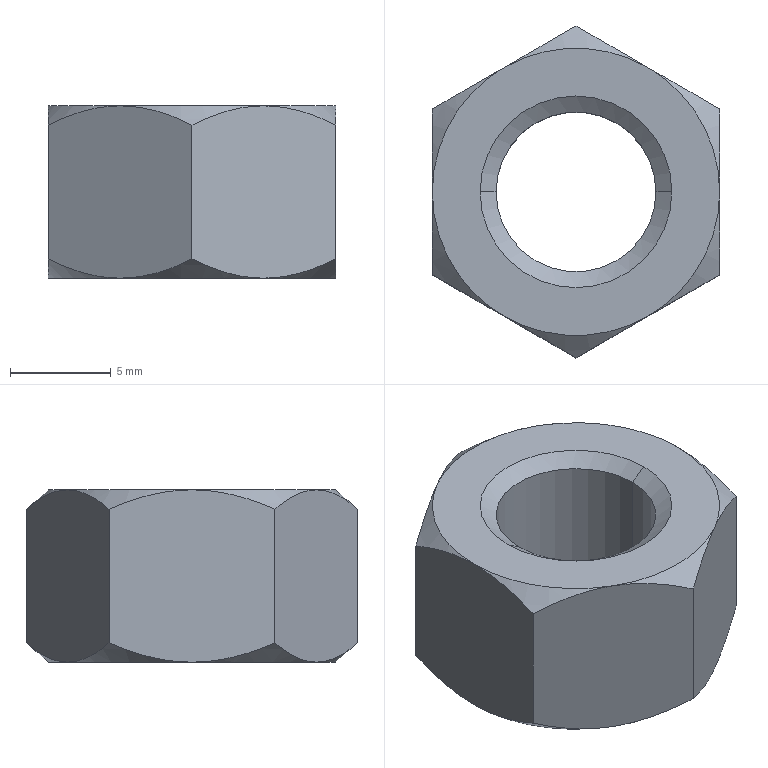Part | SolidWorks | features RevCut 4, Extrusion 1, LPattern 1 | 1 solid | 28 faces | box 14.275 x 16.483 x 8.56 mm | volume 1065 mm3 | cone 16 | plane 8 | cylinder 4 | commonest cylinder face diameters 7.938 x2 9.525 x2
STEP:
#1=CARTESIAN_POINT('',(-0.1875,0.,-0.337));
#2=VERTEX_POINT('',#1);
#3=CARTESIAN_POINT('',(0.1875,0.,-0.337));
#4=VERTEX_POINT('',#3);
#5=CARTESIAN_POINT('',(0.,0.,-0.337));
#6=DIRECTION('',(0.,0.,1.));
#7=DIRECTION('',(-1.,0.,0.));
#8=AXIS2_PLACEMENT_3D('',#5,#6,#7);
#9=CIRCLE('',#8,0.1875);
#10=EDGE_CURVE('',#2,#4,#9,.T.);
#11=ORIENTED_EDGE('',*,*,#10,.F.);
#12=CARTESIAN_POINT('',(-0.1875,0.,-0.336));
#13=VERTEX_POINT('',#12);
#14=CARTESIAN_POINT('',(-0.1875,0.,-0.9857));
#15=DIRECTION('',(0.,0.,1.));
#16=VECTOR('',#15,39.37);
#17=LINE('',#14,#16);
#18=EDGE_CURVE('',#2,#13,#17,.T.);
#19=ORIENTED_EDGE('',*,*,#18,.T.);
#20=CARTESIAN_POINT('',(0.1875,0.,-0.336));
#21=VERTEX_POINT('',#20);
#22=CARTESIAN_POINT('',(0.,0.,-0.336));
#23=DIRECTION('',(0.,0.,1.));
#24=DIRECTION('',(1.,0.,0.));
#25=AXIS2_PLACEMENT_3D('',#22,#23,#24);
#26=CIRCLE('',#25,0.1875);
#27=EDGE_CURVE('',#13,#21,#26,.T.);
#28=ORIENTED_EDGE('',*,*,#27,.T.);
#29=CARTESIAN_POINT('',(0.1875,0.,-0.9857));
#30=DIRECTION('',(0.,0.,1.));
#31=VECTOR('',#30,39.37);
#32=LINE('',#29,#31);
#33=EDGE_CURVE('',#4,#21,#32,.T.);
#34=ORIENTED_EDGE('',*,*,#33,.F.);
#35=EDGE_LOOP('',(#11,#19,#28,#34));
#36=FACE_OUTER_BOUND('',#35,.T.);
#37=CARTESIAN_POINT('',(0.,0.,-0.9857));
#38=DIRECTION('',(0.,0.,1.));
#39=DIRECTION('',(1.,0.,0.));
#40=AXIS2_PLACEMENT_3D('',#37,#38,#39);
#41=CYLINDRICAL_SURFACE('',#40,0.1875);
#42=ADVANCED_FACE('',(#36),#41,.F.);
#43=CARTESIAN_POINT('',(-0.1562,0.,-0.3141));
#44=VERTEX_POINT('',#43);
#45=CARTESIAN_POINT('',(0.1562,0.,-0.3141));
#46=VERTEX_POINT('',#45);
#47=CARTESIAN_POINT('',(0.,0.,-0.3141));
#48=DIRECTION('',(0.,0.,1.));
#49=DIRECTION('',(-1.,0.,0.));
#50=AXIS2_PLACEMENT_3D('',#47,#48,#49);
#51=CIRCLE('',#50,0.1562);
#52=EDGE_CURVE('',#44,#46,#51,.T.);
#53=ORIENTED_EDGE('',*,*,#52,.T.);
#54=CARTESIAN_POINT('',(0.1875,0.,-0.336));
#55=DIRECTION('',(0.8192,0.,-0.5736));
#56=VECTOR('',#55,39.37);
#57=LINE('',#54,#56);
#58=EDGE_CURVE('',#46,#21,#57,.T.);
#59=ORIENTED_EDGE('',*,*,#58,.T.);
#60=ORIENTED_EDGE('',*,*,#27,.F.);
#61=CARTESIAN_POINT('',(-0.1875,0.,-0.336));
#62=DIRECTION('',(-0.8192,0.,-0.5736));
#63=VECTOR('',#62,39.37);
#64=LINE('',#61,#63);
#65=EDGE_CURVE('',#44,#13,#64,.T.);
#66=ORIENTED_EDGE('',*,*,#65,.F.);
#67=EDGE_LOOP('',(#53,#59,#60,#66));
#68=FACE_OUTER_BOUND('',#67,.T.);
#69=CARTESIAN_POINT('',(0.,0.,-0.336));
#70=DIRECTION('',(0.,0.,-1.));
#71=DIRECTION('',(-1.,0.,0.));
#72=AXIS2_PLACEMENT_3D('',#69,#70,#71);
#73=CONICAL_SURFACE('',#72,0.1875,0.9599);
#74=ADVANCED_FACE('',(#68),#73,.F.);
#75=CARTESIAN_POINT('',(0.1562,0.,-0.02188));
#76=VERTEX_POINT('',#75);
#77=CARTESIAN_POINT('',(-0.1562,0.,-0.02188));
#78=VERTEX_POINT('',#77);
#79=CARTESIAN_POINT('',(0.,0.,-0.02188));
#80=DIRECTION('',(0.,0.,-1.));
#81=DIRECTION('',(1.,0.,0.));
#82=AXIS2_PLACEMENT_3D('',#79,#80,#81);
#83=CIRCLE('',#82,0.1562);
#84=EDGE_CURVE('',#76,#78,#83,.T.);
#85=ORIENTED_EDGE('',*,*,#84,.T.);
#86=CARTESIAN_POINT('',(-0.1875,0.,0.));
#87=VERTEX_POINT('',#86);
#88=CARTESIAN_POINT('',(-0.1531,0.,-0.02407));
#89=DIRECTION('',(-0.8192,0.,0.5736));
#90=VECTOR('',#89,39.37);
#91=LINE('',#88,#90);
#92=EDGE_CURVE('',#78,#87,#91,.T.);
#93=ORIENTED_EDGE('',*,*,#92,.T.);
#94=CARTESIAN_POINT('',(0.1875,0.,0.));
#95=VERTEX_POINT('',#94);
#96=CARTESIAN_POINT('',(0.,0.,0.));
#97=DIRECTION('',(0.,0.,1.));
#98=DIRECTION('',(1.,0.,0.));
#99=AXIS2_PLACEMENT_3D('',#96,#97,#98);
#100=CIRCLE('',#99,0.1875);
#101=EDGE_CURVE('',#87,#95,#100,.T.);
#102=ORIENTED_EDGE('',*,*,#101,.T.);
#103=CARTESIAN_POINT('',(0.1531,0.,-0.02407));
#104=DIRECTION('',(0.8192,0.,0.5736));
#105=VECTOR('',#104,39.37);
#106=LINE('',#103,#105);
#107=EDGE_CURVE('',#76,#95,#106,.T.);
#108=ORIENTED_EDGE('',*,*,#107,.F.);
#109=EDGE_LOOP('',(#85,#93,#102,#108));
#110=FACE_OUTER_BOUND('',#109,.T.);
#111=CARTESIAN_POINT('',(0.,0.,-0.02407));
#112=DIRECTION('',(0.,0.,1.));
#113=DIRECTION('',(1.,0.,0.));
#114=AXIS2_PLACEMENT_3D('',#111,#112,#113);
#115=CONICAL_SURFACE('',#114,0.1531,0.9599);
#116=ADVANCED_FACE('',(#110),#115,.F.);
#117=ORIENTED_EDGE('',*,*,#52,.F.);
#118=CARTESIAN_POINT('',(-0.1562,0.,-0.337));
#119=DIRECTION('',(0.,0.,1.));
#120=VECTOR('',#119,39.37);
#121=LINE('',#118,#120);
#122=EDGE_CURVE('',#44,#78,#121,.T.);
#123=ORIENTED_EDGE('',*,*,#122,.T.);
#124=ORIENTED_EDGE('',*,*,#84,.F.);
#125=CARTESIAN_POINT('',(0.1562,0.,-0.337));
#126=DIRECTION('',(0.,0.,1.));
#127=VECTOR('',#126,39.37);
#128=LINE('',#125,#127);
#129=EDGE_CURVE('',#46,#76,#128,.T.);
#130=ORIENTED_EDGE('',*,*,#129,.F.);
#131=EDGE_LOOP('',(#117,#123,#124,#130));
#132=FACE_OUTER_BOUND('',#131,.T.);
#133=CARTESIAN_POINT('',(0.,0.,-0.337));
#134=DIRECTION('',(0.,0.,1.));
#135=DIRECTION('',(1.,0.,0.));
#136=AXIS2_PLACEMENT_3D('',#133,#134,#135);
#137=CYLINDRICAL_SURFACE('',#136,0.1562);
#138=ADVANCED_FACE('',(#132),#137,.F.);
#139=ORIENTED_EDGE('',*,*,#122,.F.);
#140=CARTESIAN_POINT('',(0.,0.,-0.3141));
#141=DIRECTION('',(0.,0.,1.));
#142=DIRECTION('',(-1.,0.,0.));
#143=AXIS2_PLACEMENT_3D('',#140,#141,#142);
#144=CIRCLE('',#143,0.1562);
#145=EDGE_CURVE('',#46,#44,#144,.T.);
#146=ORIENTED_EDGE('',*,*,#145,.F.);
#147=ORIENTED_EDGE('',*,*,#129,.T.);
#148=CARTESIAN_POINT('',(0.,0.,-0.02188));
#149=DIRECTION('',(0.,0.,-1.));
#150=DIRECTION('',(1.,0.,0.));
#151=AXIS2_PLACEMENT_3D('',#148,#149,#150);
#152=CIRCLE('',#151,0.1562);
#153=EDGE_CURVE('',#78,#76,#152,.T.);
#154=ORIENTED_EDGE('',*,*,#153,.F.);
#155=EDGE_LOOP('',(#139,#146,#147,#154));
#156=FACE_OUTER_BOUND('',#155,.T.);
#157=CARTESIAN_POINT('',(0.,0.,-0.337));
#158=DIRECTION('',(0.,0.,1.));
#159=DIRECTION('',(1.,0.,0.));
#160=AXIS2_PLACEMENT_3D('',#157,#158,#159);
#161=CYLINDRICAL_SURFACE('',#160,0.1562);
#162=ADVANCED_FACE('',(#156),#161,.F.);
#163=CARTESIAN_POINT('',(-0.281,0.1622,-0.2995));
#164=VERTEX_POINT('',#163);
#165=CARTESIAN_POINT('',(-0.281,0.1622,-0.0375));
#166=VERTEX_POINT('',#165);
#167=CARTESIAN_POINT('',(-0.281,0.1622,-0.337));
#168=DIRECTION('',(0.,0.,1.));
#169=VECTOR('',#168,39.37);
#170=LINE('',#167,#169);
#171=EDGE_CURVE('',#164,#166,#170,.T.);
#172=ORIENTED_EDGE('',*,*,#171,.T.);
#173=CARTESIAN_POINT('',(-0.1405,0.2434,0.));
#174=VERTEX_POINT('',#173);
#175=CARTESIAN_POINT('',(-0.281,0.1622,-0.0375));
#176=CARTESIAN_POINT('',(-0.2586,0.1752,-0.02633));
#177=CARTESIAN_POINT('',(-0.2358,0.1883,-0.01697));
#178=CARTESIAN_POINT('',(-0.1891,0.2153,-0.003779));
#179=CARTESIAN_POINT('',(-0.1651,0.2291,0.));
#180=CARTESIAN_POINT('',(-0.1405,0.2434,0.));
#181=B_SPLINE_CURVE_WITH_KNOTS('',3,(#175,#176,#177,#178,#179,#180),.UNSPECIFIED.,.F.,.F.,(4,2,4),(0.000000248,0.002115,0.00423),.UNSPECIFIED.);
#182=EDGE_CURVE('',#166,#174,#181,.T.);
#183=ORIENTED_EDGE('',*,*,#182,.T.);
#184=CARTESIAN_POINT('',(0.,0.3245,-0.0375));
#185=VERTEX_POINT('',#184);
#186=CARTESIAN_POINT('',(-0.1405,0.2434,0.));
#187=CARTESIAN_POINT('',(-0.116,0.2575,0.));
#188=CARTESIAN_POINT('',(-0.09216,0.2713,-0.003725));
#189=CARTESIAN_POINT('',(-0.04539,0.2983,-0.01689));
#190=CARTESIAN_POINT('',(-0.02238,0.3115,-0.02635));
#191=CARTESIAN_POINT('',(0.,0.3245,-0.0375));
#192=B_SPLINE_CURVE_WITH_KNOTS('',3,(#186,#187,#188,#189,#190,#191),.UNSPECIFIED.,.F.,.F.,(4,2,4),(0.00423,0.006334,0.008438),.UNSPECIFIED.);
#193=EDGE_CURVE('',#174,#185,#192,.T.);
#194=ORIENTED_EDGE('',*,*,#193,.T.);
#195=CARTESIAN_POINT('',(0.,0.3245,-0.2995));
#196=VERTEX_POINT('',#195);
#197=CARTESIAN_POINT('',(0.,0.3245,-0.337));
#198=DIRECTION('',(0.,0.,1.));
#199=VECTOR('',#198,39.37);
#200=LINE('',#197,#199);
#201=EDGE_CURVE('',#196,#185,#200,.T.);
#202=ORIENTED_EDGE('',*,*,#201,.F.);
#203=CARTESIAN_POINT('',(-0.1405,0.2434,-0.337));
#204=VERTEX_POINT('',#203);
#205=CARTESIAN_POINT('',(-0.1405,0.2434,-0.337));
#206=CARTESIAN_POINT('',(-0.116,0.2575,-0.337));
#207=CARTESIAN_POINT('',(-0.09216,0.2713,-0.3333));
#208=CARTESIAN_POINT('',(-0.04539,0.2983,-0.3201));
#209=CARTESIAN_POINT('',(-0.02238,0.3115,-0.3106));
#210=CARTESIAN_POINT('',(0.,0.3245,-0.2995));
#211=B_SPLINE_CURVE_WITH_KNOTS('',3,(#205,#206,#207,#208,#209,#210),.UNSPECIFIED.,.F.,.F.,(4,2,4),(0.00423,0.006334,0.008438),.UNSPECIFIED.);
#212=EDGE_CURVE('',#204,#196,#211,.T.);
#213=ORIENTED_EDGE('',*,*,#212,.F.);
#214=CARTESIAN_POINT('',(-0.281,0.1622,-0.2995));
#215=CARTESIAN_POINT('',(-0.2586,0.1752,-0.3107));
#216=CARTESIAN_POINT('',(-0.2358,0.1883,-0.32));
#217=CARTESIAN_POINT('',(-0.1891,0.2153,-0.3332));
#218=CARTESIAN_POINT('',(-0.1651,0.2291,-0.337));
#219=CARTESIAN_POINT('',(-0.1405,0.2434,-0.337));
#220=B_SPLINE_CURVE_WITH_KNOTS('',3,(#214,#215,#216,#217,#218,#219),.UNSPECIFIED.,.F.,.F.,(4,2,4),(0.000000248,0.002115,0.00423),.UNSPECIFIED.);
#221=EDGE_CURVE('',#164,#204,#220,.T.);
#222=ORIENTED_EDGE('',*,*,#221,.F.);
#223=EDGE_LOOP('',(#172,#183,#194,#202,#213,#222));
#224=FACE_OUTER_BOUND('',#223,.T.);
#225=CARTESIAN_POINT('',(0.,0.3245,-0.337));
#226=DIRECTION('',(-0.5,0.866,0.));
#227=DIRECTION('',(-0.866,-0.5,0.));
#228=AXIS2_PLACEMENT_3D('',#225,#226,#227);
#229=PLANE('',#228);
#230=ADVANCED_FACE('',(#224),#229,.T.);
#231=ORIENTED_EDGE('',*,*,#201,.T.);
#232=CARTESIAN_POINT('',(0.1405,0.2434,0.));
#233=VERTEX_POINT('',#232);
#234=CARTESIAN_POINT('',(0.,0.3245,-0.0375));
#235=CARTESIAN_POINT('',(0.02242,0.3115,-0.02633));
#236=CARTESIAN_POINT('',(0.0452,0.2984,-0.01697));
#237=CARTESIAN_POINT('',(0.0919,0.2714,-0.003779));
#238=CARTESIAN_POINT('',(0.1159,0.2576,0.));
#239=CARTESIAN_POINT('',(0.1405,0.2434,0.));
#240=B_SPLINE_CURVE_WITH_KNOTS('',3,(#234,#235,#236,#237,#238,#239),.UNSPECIFIED.,.F.,.F.,(4,2,4),(0.000000248,0.002115,0.00423),.UNSPECIFIED.);
#241=EDGE_CURVE('',#185,#233,#240,.T.);
#242=ORIENTED_EDGE('',*,*,#241,.T.);
#243=CARTESIAN_POINT('',(0.281,0.1622,-0.0375));
#244=VERTEX_POINT('',#243);
#245=CARTESIAN_POINT('',(0.1405,0.2434,0.));
#246=CARTESIAN_POINT('',(0.165,0.2292,0.));
#247=CARTESIAN_POINT('',(0.1888,0.2154,-0.003725));
#248=CARTESIAN_POINT('',(0.2356,0.1884,-0.01689));
#249=CARTESIAN_POINT('',(0.2586,0.1752,-0.02635));
#250=CARTESIAN_POINT('',(0.281,0.1622,-0.0375));
#251=B_SPLINE_CURVE_WITH_KNOTS('',3,(#245,#246,#247,#248,#249,#250),.UNSPECIFIED.,.F.,.F.,(4,2,4),(0.00423,0.006334,0.008438),.UNSPECIFIED.);
#252=EDGE_CURVE('',#233,#244,#251,.T.);
#253=ORIENTED_EDGE('',*,*,#252,.T.);
#254=CARTESIAN_POINT('',(0.281,0.1622,-0.2995));
#255=VERTEX_POINT('',#254);
#256=CARTESIAN_POINT('',(0.281,0.1622,-0.337));
#257=DIRECTION('',(0.,0.,1.));
#258=VECTOR('',#257,39.37);
#259=LINE('',#256,#258);
#260=EDGE_CURVE('',#255,#244,#259,.T.);
#261=ORIENTED_EDGE('',*,*,#260,.F.);
#262=CARTESIAN_POINT('',(0.1405,0.2434,-0.337));
#263=VERTEX_POINT('',#262);
#264=CARTESIAN_POINT('',(0.1405,0.2434,-0.337));
#265=CARTESIAN_POINT('',(0.165,0.2292,-0.337));
#266=CARTESIAN_POINT('',(0.1888,0.2154,-0.3333));
#267=CARTESIAN_POINT('',(0.2356,0.1884,-0.3201));
#268=CARTESIAN_POINT('',(0.2586,0.1752,-0.3106));
#269=CARTESIAN_POINT('',(0.281,0.1622,-0.2995));
#270=B_SPLINE_CURVE_WITH_KNOTS('',3,(#264,#265,#266,#267,#268,#269),.UNSPECIFIED.,.F.,.F.,(4,2,4),(0.00423,0.006334,0.008438),.UNSPECIFIED.);
#271=EDGE_CURVE('',#263,#255,#270,.T.);
#272=ORIENTED_EDGE('',*,*,#271,.F.);
#273=CARTESIAN_POINT('',(0.,0.3245,-0.2995));
#274=CARTESIAN_POINT('',(0.02242,0.3115,-0.3107));
#275=CARTESIAN_POINT('',(0.0452,0.2984,-0.32));
#276=CARTESIAN_POINT('',(0.0919,0.2714,-0.3332));
#277=CARTESIAN_POINT('',(0.1159,0.2576,-0.337));
#278=CARTESIAN_POINT('',(0.1405,0.2434,-0.337));
#279=B_SPLINE_CURVE_WITH_KNOTS('',3,(#273,#274,#275,#276,#277,#278),.UNSPECIFIED.,.F.,.F.,(4,2,4),(0.000000248,0.002115,0.00423),.UNSPECIFIED.);
#280=EDGE_CURVE('',#196,#263,#279,.T.);
#281=ORIENTED_EDGE('',*,*,#280,.F.);
#282=EDGE_LOOP('',(#231,#242,#253,#261,#272,#281));
#283=FACE_OUTER_BOUND('',#282,.T.);
#284=CARTESIAN_POINT('',(0.281,0.1622,-0.337));
#285=DIRECTION('',(0.5,0.866,0.));
#286=DIRECTION('',(-0.866,0.5,0.));
#287=AXIS2_PLACEMENT_3D('',#284,#285,#286);
#288=PLANE('',#287);
#289=ADVANCED_FACE('',(#283),#288,.T.);
#290=CARTESIAN_POINT('',(0.281,-0.1622,-0.0375));
#291=VERTEX_POINT('',#290);
#292=CARTESIAN_POINT('',(0.281,0.,0.));
#293=VERTEX_POINT('',#292);
#294=CARTESIAN_POINT('',(0.281,-0.1622,-0.0375));
#295=CARTESIAN_POINT('',(0.281,-0.1366,-0.02645));
#296=CARTESIAN_POINT('',(0.281,-0.1099,-0.01691));
#297=CARTESIAN_POINT('',(0.281,-0.05571,-0.003699));
#298=CARTESIAN_POINT('',(0.281,-0.02815,0.));
#299=CARTESIAN_POINT('',(0.281,0.,0.));
#300=B_SPLINE_CURVE_WITH_KNOTS('',3,(#294,#295,#296,#297,#298,#299),.UNSPECIFIED.,.F.,.F.,(4,2,4),(0.005766,0.007883,0.01),.UNSPECIFIED.);
#301=EDGE_CURVE('',#291,#293,#300,.T.);
#302=ORIENTED_EDGE('',*,*,#301,.F.);
#303=CARTESIAN_POINT('',(0.281,-0.1622,-0.2995));
#304=VERTEX_POINT('',#303);
#305=CARTESIAN_POINT('',(0.281,-0.1622,-0.337));
#306=DIRECTION('',(0.,0.,1.));
#307=VECTOR('',#306,39.37);
#308=LINE('',#305,#307);
#309=EDGE_CURVE('',#304,#291,#308,.T.);
#310=ORIENTED_EDGE('',*,*,#309,.F.);
#311=CARTESIAN_POINT('',(0.281,0.,-0.337));
#312=VERTEX_POINT('',#311);
#313=CARTESIAN_POINT('',(0.281,-0.1622,-0.2995));
#314=CARTESIAN_POINT('',(0.281,-0.1366,-0.3106));
#315=CARTESIAN_POINT('',(0.281,-0.1099,-0.3201));
#316=CARTESIAN_POINT('',(0.281,-0.05571,-0.3333));
#317=CARTESIAN_POINT('',(0.281,-0.02815,-0.337));
#318=CARTESIAN_POINT('',(0.281,0.,-0.337));
#319=B_SPLINE_CURVE_WITH_KNOTS('',3,(#313,#314,#315,#316,#317,#318),.UNSPECIFIED.,.F.,.F.,(4,2,4),(0.005766,0.007883,0.01),.UNSPECIFIED.);
#320=EDGE_CURVE('',#304,#312,#319,.T.);
#321=ORIENTED_EDGE('',*,*,#320,.T.);
#322=CARTESIAN_POINT('',(0.281,0.,-0.337));
#323=CARTESIAN_POINT('',(0.281,0.01403,-0.337));
#324=CARTESIAN_POINT('',(0.281,0.02815,-0.3361));
#325=CARTESIAN_POINT('',(0.281,0.05582,-0.3325));
#326=CARTESIAN_POINT('',(0.281,0.06949,-0.3299));
#327=CARTESIAN_POINT('',(0.281,0.09651,-0.3233));
#328=CARTESIAN_POINT('',(0.281,0.1099,-0.3193));
#329=CARTESIAN_POINT('',(0.281,0.1364,-0.3102));
#330=CARTESIAN_POINT('',(0.281,0.1495,-0.305));
#331=CARTESIAN_POINT('',(0.281,0.1622,-0.2995));
#332=B_SPLINE_CURVE_WITH_KNOTS('',3,(#322,#323,#324,#325,#326,#327,#328,#329,#330,#331),.UNSPECIFIED.,.F.,.F.,(4,2,2,2,4),(0.01,0.01106,0.01211,0.01317,0.01422),.UNSPECIFIED.);
#333=EDGE_CURVE('',#312,#255,#332,.T.);
#334=ORIENTED_EDGE('',*,*,#333,.T.);
#335=ORIENTED_EDGE('',*,*,#260,.T.);
#336=CARTESIAN_POINT('',(0.281,0.,0.));
#337=CARTESIAN_POINT('',(0.281,0.01403,0.));
#338=CARTESIAN_POINT('',(0.281,0.02815,-0.0009271));
#339=CARTESIAN_POINT('',(0.281,0.05582,-0.004455));
#340=CARTESIAN_POINT('',(0.281,0.06949,-0.007051));
#341=CARTESIAN_POINT('',(0.281,0.09651,-0.01366));
#342=CARTESIAN_POINT('',(0.281,0.1099,-0.01766));
#343=CARTESIAN_POINT('',(0.281,0.1364,-0.02683));
#344=CARTESIAN_POINT('',(0.281,0.1495,-0.03199));
#345=CARTESIAN_POINT('',(0.281,0.1622,-0.0375));
#346=B_SPLINE_CURVE_WITH_KNOTS('',3,(#336,#337,#338,#339,#340,#341,#342,#343,#344,#345),.UNSPECIFIED.,.F.,.F.,(4,2,2,2,4),(0.01,0.01106,0.01211,0.01317,0.01422),.UNSPECIFIED.);
#347=EDGE_CURVE('',#293,#244,#346,.T.);
#348=ORIENTED_EDGE('',*,*,#347,.F.);
#349=EDGE_LOOP('',(#302,#310,#321,#334,#335,#348));
#350=FACE_OUTER_BOUND('',#349,.T.);
#351=CARTESIAN_POINT('',(0.281,0.1622,-0.337));
#352=DIRECTION('',(-1.,0.,0.));
#353=DIRECTION('',(0.,0.,1.));
#354=AXIS2_PLACEMENT_3D('',#351,#352,#353);
#355=PLANE('',#354);
#356=ADVANCED_FACE('',(#350),#355,.F.);
#357=ORIENTED_EDGE('',*,*,#309,.T.);
#358=CARTESIAN_POINT('',(0.1405,-0.2434,0.));
#359=VERTEX_POINT('',#358);
#360=CARTESIAN_POINT('',(0.281,-0.1622,-0.0375));
#361=CARTESIAN_POINT('',(0.2586,-0.1752,-0.02633));
#362=CARTESIAN_POINT('',(0.2358,-0.1883,-0.01697));
#363=CARTESIAN_POINT('',(0.1891,-0.2153,-0.003779));
#364=CARTESIAN_POINT('',(0.1651,-0.2291,0.));
#365=CARTESIAN_POINT('',(0.1405,-0.2434,0.));
#366=B_SPLINE_CURVE_WITH_KNOTS('',3,(#360,#361,#362,#363,#364,#365),.UNSPECIFIED.,.F.,.F.,(4,2,4),(0.000000248,0.002115,0.00423),.UNSPECIFIED.);
#367=EDGE_CURVE('',#291,#359,#366,.T.);
#368=ORIENTED_EDGE('',*,*,#367,.T.);
#369=CARTESIAN_POINT('',(0.,-0.3245,-0.0375));
#370=VERTEX_POINT('',#369);
#371=CARTESIAN_POINT('',(0.1405,-0.2434,0.));
#372=CARTESIAN_POINT('',(0.116,-0.2575,0.));
#373=CARTESIAN_POINT('',(0.09216,-0.2713,-0.003725));
#374=CARTESIAN_POINT('',(0.04539,-0.2983,-0.01689));
#375=CARTESIAN_POINT('',(0.02238,-0.3115,-0.02635));
#376=CARTESIAN_POINT('',(0.,-0.3245,-0.0375));
#377=B_SPLINE_CURVE_WITH_KNOTS('',3,(#371,#372,#373,#374,#375,#376),.UNSPECIFIED.,.F.,.F.,(4,2,4),(0.00423,0.006334,0.008438),.UNSPECIFIED.);
#378=EDGE_CURVE('',#359,#370,#377,.T.);
#379=ORIENTED_EDGE('',*,*,#378,.T.);
#380=CARTESIAN_POINT('',(0.,-0.3245,-0.2995));
#381=VERTEX_POINT('',#380);
#382=CARTESIAN_POINT('',(0.,-0.3245,-0.337));
#383=DIRECTION('',(0.,0.,1.));
#384=VECTOR('',#383,39.37);
#385=LINE('',#382,#384);
#386=EDGE_CURVE('',#381,#370,#385,.T.);
#387=ORIENTED_EDGE('',*,*,#386,.F.);
#388=CARTESIAN_POINT('',(0.1405,-0.2434,-0.337));
#389=VERTEX_POINT('',#388);
#390=CARTESIAN_POINT('',(0.1405,-0.2434,-0.337));
#391=CARTESIAN_POINT('',(0.116,-0.2575,-0.337));
#392=CARTESIAN_POINT('',(0.09216,-0.2713,-0.3333));
#393=CARTESIAN_POINT('',(0.04539,-0.2983,-0.3201));
#394=CARTESIAN_POINT('',(0.02238,-0.3115,-0.3106));
#395=CARTESIAN_POINT('',(0.,-0.3245,-0.2995));
#396=B_SPLINE_CURVE_WITH_KNOTS('',3,(#390,#391,#392,#393,#394,#395),.UNSPECIFIED.,.F.,.F.,(4,2,4),(0.00423,0.006334,0.008438),.UNSPECIFIED.);
#397=EDGE_CURVE('',#389,#381,#396,.T.);
#398=ORIENTED_EDGE('',*,*,#397,.F.);
#399=CARTESIAN_POINT('',(0.281,-0.1622,-0.2995));
#400=CARTESIAN_POINT('',(0.2586,-0.1752,-0.3107));
#401=CARTESIAN_POINT('',(0.2358,-0.1883,-0.32));
#402=CARTESIAN_POINT('',(0.1891,-0.2153,-0.3332));
#403=CARTESIAN_POINT('',(0.1651,-0.2291,-0.337));
#404=CARTESIAN_POINT('',(0.1405,-0.2434,-0.337));
#405=B_SPLINE_CURVE_WITH_KNOTS('',3,(#399,#400,#401,#402,#403,#404),.UNSPECIFIED.,.F.,.F.,(4,2,4),(0.000000248,0.002115,0.00423),.UNSPECIFIED.);
#406=EDGE_CURVE('',#304,#389,#405,.T.);
#407=ORIENTED_EDGE('',*,*,#406,.F.);
#408=EDGE_LOOP('',(#357,#368,#379,#387,#398,#407));
#409=FACE_OUTER_BOUND('',#408,.T.);
#410=CARTESIAN_POINT('',(0.,-0.3245,-0.337));
#411=DIRECTION('',(0.5,-0.866,0.));
#412=DIRECTION('',(0.866,0.5,0.));
#413=AXIS2_PLACEMENT_3D('',#410,#411,#412);
#414=PLANE('',#413);
#415=ADVANCED_FACE('',(#409),#414,.T.);
#416=ORIENTED_EDGE('',*,*,#386,.T.);
#417=CARTESIAN_POINT('',(-0.1405,-0.2434,0.));
#418=VERTEX_POINT('',#417);
#419=CARTESIAN_POINT('',(0.,-0.3245,-0.0375));
#420=CARTESIAN_POINT('',(-0.02242,-0.3115,-0.02633));
#421=CARTESIAN_POINT('',(-0.0452,-0.2984,-0.01697));
#422=CARTESIAN_POINT('',(-0.0919,-0.2714,-0.003779));
#423=CARTESIAN_POINT('',(-0.1159,-0.2576,0.));
#424=CARTESIAN_POINT('',(-0.1405,-0.2434,0.));
#425=B_SPLINE_CURVE_WITH_KNOTS('',3,(#419,#420,#421,#422,#423,#424),.UNSPECIFIED.,.F.,.F.,(4,2,4),(0.000000248,0.002115,0.00423),.UNSPECIFIED.);
#426=EDGE_CURVE('',#370,#418,#425,.T.);
#427=ORIENTED_EDGE('',*,*,#426,.T.);
#428=CARTESIAN_POINT('',(-0.281,-0.1622,-0.0375));
#429=VERTEX_POINT('',#428);
#430=CARTESIAN_POINT('',(-0.1405,-0.2434,0.));
#431=CARTESIAN_POINT('',(-0.165,-0.2292,0.));
#432=CARTESIAN_POINT('',(-0.1888,-0.2154,-0.003725));
#433=CARTESIAN_POINT('',(-0.2356,-0.1884,-0.01689));
#434=CARTESIAN_POINT('',(-0.2586,-0.1752,-0.02635));
#435=CARTESIAN_POINT('',(-0.281,-0.1622,-0.0375));
#436=B_SPLINE_CURVE_WITH_KNOTS('',3,(#430,#431,#432,#433,#434,#435),.UNSPECIFIED.,.F.,.F.,(4,2,4),(0.00423,0.006334,0.008438),.UNSPECIFIED.);
#437=EDGE_CURVE('',#418,#429,#436,.T.);
#438=ORIENTED_EDGE('',*,*,#437,.T.);
#439=CARTESIAN_POINT('',(-0.281,-0.1622,-0.2995));
#440=VERTEX_POINT('',#439);
#441=CARTESIAN_POINT('',(-0.281,-0.1622,-0.337));
#442=DIRECTION('',(0.,0.,1.));
#443=VECTOR('',#442,39.37);
#444=LINE('',#441,#443);
#445=EDGE_CURVE('',#440,#429,#444,.T.);
#446=ORIENTED_EDGE('',*,*,#445,.F.);
#447=CARTESIAN_POINT('',(-0.1405,-0.2434,-0.337));
#448=VERTEX_POINT('',#447);
#449=CARTESIAN_POINT('',(-0.1405,-0.2434,-0.337));
#450=CARTESIAN_POINT('',(-0.165,-0.2292,-0.337));
#451=CARTESIAN_POINT('',(-0.1888,-0.2154,-0.3333));
#452=CARTESIAN_POINT('',(-0.2356,-0.1884,-0.3201));
#453=CARTESIAN_POINT('',(-0.2586,-0.1752,-0.3106));
#454=CARTESIAN_POINT('',(-0.281,-0.1622,-0.2995));
#455=B_SPLINE_CURVE_WITH_KNOTS('',3,(#449,#450,#451,#452,#453,#454),.UNSPECIFIED.,.F.,.F.,(4,2,4),(0.00423,0.006334,0.008438),.UNSPECIFIED.);
#456=EDGE_CURVE('',#448,#440,#455,.T.);
#457=ORIENTED_EDGE('',*,*,#456,.F.);
#458=CARTESIAN_POINT('',(0.,-0.3245,-0.2995));
#459=CARTESIAN_POINT('',(-0.02242,-0.3115,-0.3107));
#460=CARTESIAN_POINT('',(-0.0452,-0.2984,-0.32));
#461=CARTESIAN_POINT('',(-0.0919,-0.2714,-0.3332));
#462=CARTESIAN_POINT('',(-0.1159,-0.2576,-0.337));
#463=CARTESIAN_POINT('',(-0.1405,-0.2434,-0.337));
#464=B_SPLINE_CURVE_WITH_KNOTS('',3,(#458,#459,#460,#461,#462,#463),.UNSPECIFIED.,.F.,.F.,(4,2,4),(0.000000248,0.002115,0.00423),.UNSPECIFIED.);
#465=EDGE_CURVE('',#381,#448,#464,.T.);
#466=ORIENTED_EDGE('',*,*,#465,.F.);
#467=EDGE_LOOP('',(#416,#427,#438,#446,#457,#466));
#468=FACE_OUTER_BOUND('',#467,.T.);
#469=CARTESIAN_POINT('',(-0.281,-0.1622,-0.337));
#470=DIRECTION('',(-0.5,-0.866,0.));
#471=DIRECTION('',(0.866,-0.5,0.));
#472=AXIS2_PLACEMENT_3D('',#469,#470,#471);
#473=PLANE('',#472);
#474=ADVANCED_FACE('',(#468),#473,.T.);
#475=ORIENTED_EDGE('',*,*,#445,.T.);
#476=CARTESIAN_POINT('',(-0.281,0.,0.));
#477=VERTEX_POINT('',#476);
#478=CARTESIAN_POINT('',(-0.281,-0.1622,-0.0375));
#479=CARTESIAN_POINT('',(-0.281,-0.1366,-0.02645));
#480=CARTESIAN_POINT('',(-0.281,-0.1099,-0.01691));
#481=CARTESIAN_POINT('',(-0.281,-0.05571,-0.003699));
#482=CARTESIAN_POINT('',(-0.281,-0.02815,0.));
#483=CARTESIAN_POINT('',(-0.281,0.,0.));
#484=B_SPLINE_CURVE_WITH_KNOTS('',3,(#478,#479,#480,#481,#482,#483),.UNSPECIFIED.,.F.,.F.,(4,2,4),(0.005766,0.007883,0.01),.UNSPECIFIED.);
#485=EDGE_CURVE('',#429,#477,#484,.T.);
#486=ORIENTED_EDGE('',*,*,#485,.T.);
#487=CARTESIAN_POINT('',(-0.281,0.,0.));
#488=CARTESIAN_POINT('',(-0.281,0.01403,0.));
#489=CARTESIAN_POINT('',(-0.281,0.02815,-0.0009271));
#490=CARTESIAN_POINT('',(-0.281,0.05582,-0.004455));
#491=CARTESIAN_POINT('',(-0.281,0.06949,-0.007051));
#492=CARTESIAN_POINT('',(-0.281,0.09651,-0.01366));
#493=CARTESIAN_POINT('',(-0.281,0.1099,-0.01766));
#494=CARTESIAN_POINT('',(-0.281,0.1364,-0.02683));
#495=CARTESIAN_POINT('',(-0.281,0.1495,-0.03199));
#496=CARTESIAN_POINT('',(-0.281,0.1622,-0.0375));
#497=B_SPLINE_CURVE_WITH_KNOTS('',3,(#487,#488,#489,#490,#491,#492,#493,#494,#495,#496),.UNSPECIFIED.,.F.,.F.,(4,2,2,2,4),(0.01,0.01106,0.01211,0.01317,0.01422),.UNSPECIFIED.);
#498=EDGE_CURVE('',#477,#166,#497,.T.);
#499=ORIENTED_EDGE('',*,*,#498,.T.);
#500=ORIENTED_EDGE('',*,*,#171,.F.);
#501=CARTESIAN_POINT('',(-0.281,0.,-0.337));
#502=VERTEX_POINT('',#501);
#503=CARTESIAN_POINT('',(-0.281,0.,-0.337));
#504=CARTESIAN_POINT('',(-0.281,0.01403,-0.337));
#505=CARTESIAN_POINT('',(-0.281,0.02815,-0.3361));
#506=CARTESIAN_POINT('',(-0.281,0.05582,-0.3325));
#507=CARTESIAN_POINT('',(-0.281,0.06949,-0.3299));
#508=CARTESIAN_POINT('',(-0.281,0.09651,-0.3233));
#509=CARTESIAN_POINT('',(-0.281,0.1099,-0.3193));
#510=CARTESIAN_POINT('',(-0.281,0.1364,-0.3102));
#511=CARTESIAN_POINT('',(-0.281,0.1495,-0.305));
#512=CARTESIAN_POINT('',(-0.281,0.1622,-0.2995));
#513=B_SPLINE_CURVE_WITH_KNOTS('',3,(#503,#504,#505,#506,#507,#508,#509,#510,#511,#512),.UNSPECIFIED.,.F.,.F.,(4,2,2,2,4),(0.01,0.01106,0.01211,0.01317,0.01422),.UNSPECIFIED.);
#514=EDGE_CURVE('',#502,#164,#513,.T.);
#515=ORIENTED_EDGE('',*,*,#514,.F.);
#516=CARTESIAN_POINT('',(-0.281,-0.1622,-0.2995));
#517=CARTESIAN_POINT('',(-0.281,-0.1366,-0.3106));
#518=CARTESIAN_POINT('',(-0.281,-0.1099,-0.3201));
#519=CARTESIAN_POINT('',(-0.281,-0.05571,-0.3333));
#520=CARTESIAN_POINT('',(-0.281,-0.02815,-0.337));
#521=CARTESIAN_POINT('',(-0.281,0.,-0.337));
#522=B_SPLINE_CURVE_WITH_KNOTS('',3,(#516,#517,#518,#519,#520,#521),.UNSPECIFIED.,.F.,.F.,(4,2,4),(0.005766,0.007883,0.01),.UNSPECIFIED.);
#523=EDGE_CURVE('',#440,#502,#522,.T.);
#524=ORIENTED_EDGE('',*,*,#523,.F.);
#525=EDGE_LOOP('',(#475,#486,#499,#500,#515,#524));
#526=FACE_OUTER_BOUND('',#525,.T.);
#527=CARTESIAN_POINT('',(-0.281,0.1622,-0.337));
#528=DIRECTION('',(-1.,0.,0.));
#529=DIRECTION('',(0.,0.,1.));
#530=AXIS2_PLACEMENT_3D('',#527,#528,#529);
#531=PLANE('',#530);
#532=ADVANCED_FACE('',(#526),#531,.T.);
#533=CARTESIAN_POINT('',(0.,0.,0.));
#534=DIRECTION('',(0.,0.,1.));
#535=DIRECTION('',(1.,0.,0.));
#536=AXIS2_PLACEMENT_3D('',#533,#534,#535);
#537=CIRCLE('',#536,0.1875);
#538=EDGE_CURVE('',#95,#87,#537,.T.);
#539=ORIENTED_EDGE('',*,*,#538,.F.);
#540=ORIENTED_EDGE('',*,*,#101,.F.);
#541=EDGE_LOOP('',(#539,#540));
#542=FACE_BOUND('',#541,.T.);
#543=CARTESIAN_POINT('',(0.,0.,0.));
#544=DIRECTION('',(0.,0.,-1.));
#545=DIRECTION('',(-1.,0.,0.));
#546=AXIS2_PLACEMENT_3D('',#543,#544,#545);
#547=CIRCLE('',#546,0.281);
#548=EDGE_CURVE('',#477,#174,#547,.T.);
#549=ORIENTED_EDGE('',*,*,#548,.F.);
#550=CARTESIAN_POINT('',(0.,0.,0.));
#551=DIRECTION('',(0.,0.,-1.));
#552=DIRECTION('',(-1.,0.,0.));
#553=AXIS2_PLACEMENT_3D('',#550,#551,#552);
#554=CIRCLE('',#553,0.281);
#555=EDGE_CURVE('',#418,#477,#554,.T.);
#556=ORIENTED_EDGE('',*,*,#555,.F.);
#557=CARTESIAN_POINT('',(0.,0.,0.));
#558=DIRECTION('',(0.,0.,-1.));
#559=DIRECTION('',(-1.,0.,0.));
#560=AXIS2_PLACEMENT_3D('',#557,#558,#559);
#561=CIRCLE('',#560,0.281);
#562=EDGE_CURVE('',#359,#418,#561,.T.);
#563=ORIENTED_EDGE('',*,*,#562,.F.);
#564=CARTESIAN_POINT('',(0.,0.,0.));
#565=DIRECTION('',(0.,0.,-1.));
#566=DIRECTION('',(-1.,0.,0.));
#567=AXIS2_PLACEMENT_3D('',#564,#565,#566);
#568=CIRCLE('',#567,0.281);
#569=EDGE_CURVE('',#293,#359,#568,.T.);
#570=ORIENTED_EDGE('',*,*,#569,.F.);
#571=CARTESIAN_POINT('',(0.,0.,0.));
#572=DIRECTION('',(0.,0.,1.));
#573=DIRECTION('',(1.,0.,0.));
#574=AXIS2_PLACEMENT_3D('',#571,#572,#573);
#575=CIRCLE('',#574,0.281);
#576=EDGE_CURVE('',#293,#233,#575,.T.);
#577=ORIENTED_EDGE('',*,*,#576,.T.);
#578=CARTESIAN_POINT('',(0.,0.,0.));
#579=DIRECTION('',(0.,0.,-1.));
#580=DIRECTION('',(-1.,0.,0.));
#581=AXIS2_PLACEMENT_3D('',#578,#579,#580);
#582=CIRCLE('',#581,0.281);
#583=EDGE_CURVE('',#174,#233,#582,.T.);
#584=ORIENTED_EDGE('',*,*,#583,.F.);
#585=EDGE_LOOP('',(#549,#556,#563,#570,#577,#584));
#586=FACE_OUTER_BOUND('',#585,.T.);
#587=CARTESIAN_POINT('',(0.,0.3245,0.));
#588=DIRECTION('',(0.,0.,-1.));
#589=DIRECTION('',(-1.,0.,0.));
#590=AXIS2_PLACEMENT_3D('',#587,#588,#589);
#591=PLANE('',#590);
#592=ADVANCED_FACE('',(#542,#586),#591,.F.);
#593=CARTESIAN_POINT('',(0.,0.,-0.337));
#594=DIRECTION('',(0.,0.,1.));
#595=DIRECTION('',(-1.,0.,0.));
#596=AXIS2_PLACEMENT_3D('',#593,#594,#595);
#597=CIRCLE('',#596,0.1875);
#598=EDGE_CURVE('',#4,#2,#597,.T.);
#599=ORIENTED_EDGE('',*,*,#598,.T.);
#600=ORIENTED_EDGE('',*,*,#10,.T.);
#601=EDGE_LOOP('',(#599,#600));
#602=FACE_BOUND('',#601,.T.);
#603=CARTESIAN_POINT('',(0.,0.,-0.337));
#604=DIRECTION('',(0.,0.,1.));
#605=DIRECTION('',(-1.,0.,0.));
#606=AXIS2_PLACEMENT_3D('',#603,#604,#605);
#607=CIRCLE('',#606,0.281);
#608=EDGE_CURVE('',#502,#448,#607,.T.);
#609=ORIENTED_EDGE('',*,*,#608,.F.);
#610=CARTESIAN_POINT('',(0.,0.,-0.337));
#611=DIRECTION('',(0.,0.,1.));
#612=DIRECTION('',(-1.,0.,0.));
#613=AXIS2_PLACEMENT_3D('',#610,#611,#612);
#614=CIRCLE('',#613,0.281);
#615=EDGE_CURVE('',#204,#502,#614,.T.);
#616=ORIENTED_EDGE('',*,*,#615,.F.);
#617=CARTESIAN_POINT('',(0.,0.,-0.337));
#618=DIRECTION('',(0.,0.,1.));
#619=DIRECTION('',(-1.,0.,0.));
#620=AXIS2_PLACEMENT_3D('',#617,#618,#619);
#621=CIRCLE('',#620,0.281);
#622=EDGE_CURVE('',#263,#204,#621,.T.);
#623=ORIENTED_EDGE('',*,*,#622,.F.);
#624=CARTESIAN_POINT('',(0.,0.,-0.337));
#625=DIRECTION('',(0.,0.,1.));
#626=DIRECTION('',(1.,0.,0.));
#627=AXIS2_PLACEMENT_3D('',#624,#625,#626);
#628=CIRCLE('',#627,0.281);
#629=EDGE_CURVE('',#312,#263,#628,.T.);
#630=ORIENTED_EDGE('',*,*,#629,.F.);
#631=CARTESIAN_POINT('',(0.,0.,-0.337));
#632=DIRECTION('',(0.,0.,1.));
#633=DIRECTION('',(-1.,0.,0.));
#634=AXIS2_PLACEMENT_3D('',#631,#632,#633);
#635=CIRCLE('',#634,0.281);
#636=EDGE_CURVE('',#389,#312,#635,.T.);
#637=ORIENTED_EDGE('',*,*,#636,.F.);
#638=CARTESIAN_POINT('',(0.,0.,-0.337));
#639=DIRECTION('',(0.,0.,1.));
#640=DIRECTION('',(-1.,0.,0.));
#641=AXIS2_PLACEMENT_3D('',#638,#639,#640);
#642=CIRCLE('',#641,0.281);
#643=EDGE_CURVE('',#448,#389,#642,.T.);
#644=ORIENTED_EDGE('',*,*,#643,.F.);
#645=EDGE_LOOP('',(#609,#616,#623,#630,#637,#644));
#646=FACE_OUTER_BOUND('',#645,.T.);
#647=CARTESIAN_POINT('',(0.,0.3245,-0.337));
#648=DIRECTION('',(0.,0.,-1.));
#649=DIRECTION('',(-1.,0.,0.));
#650=AXIS2_PLACEMENT_3D('',#647,#648,#649);
#651=PLANE('',#650);
#652=ADVANCED_FACE('',(#602,#646),#651,.T.);
#653=ORIENTED_EDGE('',*,*,#221,.T.);
#654=ORIENTED_EDGE('',*,*,#615,.T.);
#655=ORIENTED_EDGE('',*,*,#514,.T.);
#656=EDGE_LOOP('',(#653,#654,#655));
#657=FACE_OUTER_BOUND('',#656,.T.);
#658=CARTESIAN_POINT('',(0.,0.,-0.337));
#659=DIRECTION('',(0.,0.,1.));
#660=DIRECTION('',(1.,0.,0.));
#661=AXIS2_PLACEMENT_3D('',#658,#659,#660);
#662=CONICAL_SURFACE('',#661,0.281,0.859);
#663=ADVANCED_FACE('',(#657),#662,.T.);
#664=ORIENTED_EDGE('',*,*,#212,.T.);
#665=ORIENTED_EDGE('',*,*,#280,.T.);
#666=ORIENTED_EDGE('',*,*,#622,.T.);
#667=EDGE_LOOP('',(#664,#665,#666));
#668=FACE_OUTER_BOUND('',#667,.T.);
#669=CARTESIAN_POINT('',(0.,0.,-0.337));
#670=DIRECTION('',(0.,0.,1.));
#671=DIRECTION('',(1.,0.,0.));
#672=AXIS2_PLACEMENT_3D('',#669,#670,#671);
#673=CONICAL_SURFACE('',#672,0.281,0.859);
#674=ADVANCED_FACE('',(#668),#673,.T.);
#675=ORIENTED_EDGE('',*,*,#271,.T.);
#676=ORIENTED_EDGE('',*,*,#333,.F.);
#677=ORIENTED_EDGE('',*,*,#629,.T.);
#678=EDGE_LOOP('',(#675,#676,#677));
#679=FACE_OUTER_BOUND('',#678,.T.);
#680=CARTESIAN_POINT('',(0.,0.,-0.337));
#681=DIRECTION('',(0.,0.,1.));
#682=DIRECTION('',(1.,0.,0.));
#683=AXIS2_PLACEMENT_3D('',#680,#681,#682);
#684=CONICAL_SURFACE('',#683,0.281,0.859);
#685=ADVANCED_FACE('',(#679),#684,.T.);
#686=ORIENTED_EDGE('',*,*,#406,.T.);
#687=ORIENTED_EDGE('',*,*,#636,.T.);
#688=ORIENTED_EDGE('',*,*,#320,.F.);
#689=EDGE_LOOP('',(#686,#687,#688));
#690=FACE_OUTER_BOUND('',#689,.T.);
#691=CARTESIAN_POINT('',(0.,0.,-0.337));
#692=DIRECTION('',(0.,0.,1.));
#693=DIRECTION('',(1.,0.,0.));
#694=AXIS2_PLACEMENT_3D('',#691,#692,#693);
#695=CONICAL_SURFACE('',#694,0.281,0.859);
#696=ADVANCED_FACE('',(#690),#695,.T.);
#697=ORIENTED_EDGE('',*,*,#397,.T.);
#698=ORIENTED_EDGE('',*,*,#465,.T.);
#699=ORIENTED_EDGE('',*,*,#643,.T.);
#700=EDGE_LOOP('',(#697,#698,#699));
#701=FACE_OUTER_BOUND('',#700,.T.);
#702=CARTESIAN_POINT('',(0.,0.,-0.337));
#703=DIRECTION('',(0.,0.,1.));
#704=DIRECTION('',(1.,0.,0.));
#705=AXIS2_PLACEMENT_3D('',#702,#703,#704);
#706=CONICAL_SURFACE('',#705,0.281,0.859);
#707=ADVANCED_FACE('',(#701),#706,.T.);
#708=ORIENTED_EDGE('',*,*,#456,.T.);
#709=ORIENTED_EDGE('',*,*,#523,.T.);
#710=ORIENTED_EDGE('',*,*,#608,.T.);
#711=EDGE_LOOP('',(#708,#709,#710));
#712=FACE_OUTER_BOUND('',#711,.T.);
#713=CARTESIAN_POINT('',(0.,0.,-0.337));
#714=DIRECTION('',(0.,0.,1.));
#715=DIRECTION('',(1.,0.,0.));
#716=AXIS2_PLACEMENT_3D('',#713,#714,#715);
#717=CONICAL_SURFACE('',#716,0.281,0.859);
#718=ADVANCED_FACE('',(#712),#717,.T.);
#719=ORIENTED_EDGE('',*,*,#555,.T.);
#720=ORIENTED_EDGE('',*,*,#485,.F.);
#721=ORIENTED_EDGE('',*,*,#437,.F.);
#722=EDGE_LOOP('',(#719,#720,#721));
#723=FACE_OUTER_BOUND('',#722,.T.);
#724=CARTESIAN_POINT('',(0.,0.,0.));
#725=DIRECTION('',(0.,0.,-1.));
#726=DIRECTION('',(-1.,0.,0.));
#727=AXIS2_PLACEMENT_3D('',#724,#725,#726);
#728=CONICAL_SURFACE('',#727,0.281,0.859);
#729=ADVANCED_FACE('',(#723),#728,.T.);
#730=ORIENTED_EDGE('',*,*,#562,.T.);
#731=ORIENTED_EDGE('',*,*,#426,.F.);
#732=ORIENTED_EDGE('',*,*,#378,.F.);
#733=EDGE_LOOP('',(#730,#731,#732));
#734=FACE_OUTER_BOUND('',#733,.T.);
#735=CARTESIAN_POINT('',(0.,0.,0.));
#736=DIRECTION('',(0.,0.,-1.));
#737=DIRECTION('',(-1.,0.,0.));
#738=AXIS2_PLACEMENT_3D('',#735,#736,#737);
#739=CONICAL_SURFACE('',#738,0.281,0.859);
#740=ADVANCED_FACE('',(#734),#739,.T.);
#741=ORIENTED_EDGE('',*,*,#301,.T.);
#742=ORIENTED_EDGE('',*,*,#569,.T.);
#743=ORIENTED_EDGE('',*,*,#367,.F.);
#744=EDGE_LOOP('',(#741,#742,#743));
#745=FACE_OUTER_BOUND('',#744,.T.);
#746=CARTESIAN_POINT('',(0.,0.,0.));
#747=DIRECTION('',(0.,0.,-1.));
#748=DIRECTION('',(-1.,0.,0.));
#749=AXIS2_PLACEMENT_3D('',#746,#747,#748);
#750=CONICAL_SURFACE('',#749,0.281,0.859);
#751=ADVANCED_FACE('',(#745),#750,.T.);
#752=ORIENTED_EDGE('',*,*,#576,.F.);
#753=ORIENTED_EDGE('',*,*,#347,.T.);
#754=ORIENTED_EDGE('',*,*,#252,.F.);
#755=EDGE_LOOP('',(#752,#753,#754));
#756=FACE_OUTER_BOUND('',#755,.T.);
#757=CARTESIAN_POINT('',(0.,0.,0.));
#758=DIRECTION('',(0.,0.,-1.));
#759=DIRECTION('',(-1.,0.,0.));
#760=AXIS2_PLACEMENT_3D('',#757,#758,#759);
#761=CONICAL_SURFACE('',#760,0.281,0.859);
#762=ADVANCED_FACE('',(#756),#761,.T.);
#763=ORIENTED_EDGE('',*,*,#583,.T.);
#764=ORIENTED_EDGE('',*,*,#241,.F.);
#765=ORIENTED_EDGE('',*,*,#193,.F.);
#766=EDGE_LOOP('',(#763,#764,#765));
#767=FACE_OUTER_BOUND('',#766,.T.);
#768=CARTESIAN_POINT('',(0.,0.,0.));
#769=DIRECTION('',(0.,0.,-1.));
#770=DIRECTION('',(-1.,0.,0.));
#771=AXIS2_PLACEMENT_3D('',#768,#769,#770);
#772=CONICAL_SURFACE('',#771,0.281,0.859);
#773=ADVANCED_FACE('',(#767),#772,.T.);
#774=ORIENTED_EDGE('',*,*,#498,.F.);
#775=ORIENTED_EDGE('',*,*,#548,.T.);
#776=ORIENTED_EDGE('',*,*,#182,.F.);
#777=EDGE_LOOP('',(#774,#775,#776));
#778=FACE_OUTER_BOUND('',#777,.T.);
#779=CARTESIAN_POINT('',(0.,0.,0.));
#780=DIRECTION('',(0.,0.,-1.));
#781=DIRECTION('',(-1.,0.,0.));
#782=AXIS2_PLACEMENT_3D('',#779,#780,#781);
#783=CONICAL_SURFACE('',#782,0.281,0.859);
#784=ADVANCED_FACE('',(#778),#783,.T.);
#785=ORIENTED_EDGE('',*,*,#92,.F.);
#786=ORIENTED_EDGE('',*,*,#153,.T.);
#787=ORIENTED_EDGE('',*,*,#107,.T.);
#788=ORIENTED_EDGE('',*,*,#538,.T.);
#789=EDGE_LOOP('',(#785,#786,#787,#788));
#790=FACE_OUTER_BOUND('',#789,.T.);
#791=CARTESIAN_POINT('',(0.,0.,-0.02407));
#792=DIRECTION('',(0.,0.,1.));
#793=DIRECTION('',(1.,0.,0.));
#794=AXIS2_PLACEMENT_3D('',#791,#792,#793);
#795=CONICAL_SURFACE('',#794,0.1531,0.9599);
#796=ADVANCED_FACE('',(#790),#795,.F.);
#797=ORIENTED_EDGE('',*,*,#58,.F.);
#798=ORIENTED_EDGE('',*,*,#145,.T.);
#799=ORIENTED_EDGE('',*,*,#65,.T.);
#800=CARTESIAN_POINT('',(0.,0.,-0.336));
#801=DIRECTION('',(0.,0.,1.));
#802=DIRECTION('',(1.,0.,0.));
#803=AXIS2_PLACEMENT_3D('',#800,#801,#802);
#804=CIRCLE('',#803,0.1875);
#805=EDGE_CURVE('',#21,#13,#804,.T.);
#806=ORIENTED_EDGE('',*,*,#805,.F.);
#807=EDGE_LOOP('',(#797,#798,#799,#806));
#808=FACE_OUTER_BOUND('',#807,.T.);
#809=CARTESIAN_POINT('',(0.,0.,-0.336));
#810=DIRECTION('',(0.,0.,-1.));
#811=DIRECTION('',(-1.,0.,0.));
#812=AXIS2_PLACEMENT_3D('',#809,#810,#811);
#813=CONICAL_SURFACE('',#812,0.1875,0.9599);
#814=ADVANCED_FACE('',(#808),#813,.F.);
#815=ORIENTED_EDGE('',*,*,#18,.F.);
#816=ORIENTED_EDGE('',*,*,#598,.F.);
#817=ORIENTED_EDGE('',*,*,#33,.T.);
#818=ORIENTED_EDGE('',*,*,#805,.T.);
#819=EDGE_LOOP('',(#815,#816,#817,#818));
#820=FACE_OUTER_BOUND('',#819,.T.);
#821=CARTESIAN_POINT('',(0.,0.,-0.9857));
#822=DIRECTION('',(0.,0.,1.));
#823=DIRECTION('',(1.,0.,0.));
#824=AXIS2_PLACEMENT_3D('',#821,#822,#823);
#825=CYLINDRICAL_SURFACE('',#824,0.1875);
#826=ADVANCED_FACE('',(#820),#825,.F.);
#827=CLOSED_SHELL('',(#42,#74,#116,#138,#162,#230,#289,#356,#415,#474,#532,#592,#652,#663,#674,#685,#696,#707,#718,#729,#740,#751,#762,#773,#784,#796,#814,#826));
#828=MANIFOLD_SOLID_BREP('',#827);
#829=CARTESIAN_POINT('',(0.,0.,0.));
#830=DIRECTION('',(0.,0.,1.));
#831=DIRECTION('',(1.,0.,0.));
#832=AXIS2_PLACEMENT_3D('',#829,#830,#831);
#833=(LENGTH_UNIT()NAMED_UNIT(*)SI_UNIT($,.METRE.));
#834=LENGTH_MEASURE_WITH_UNIT(LENGTH_MEASURE(0.0254),#833);
#835=DIMENSIONAL_EXPONENTS(1.,0.,0.,0.,0.,0.,0.);
#836=(CONVERSION_BASED_UNIT('INCH',#834)LENGTH_UNIT()NAMED_UNIT(#835));
#837=UNCERTAINTY_MEASURE_WITH_UNIT(LENGTH_MEASURE(0.00001),#836,'','');
#838=(NAMED_UNIT(*)PLANE_ANGLE_UNIT()SI_UNIT($,.RADIAN.));
#839=(NAMED_UNIT(*)SI_UNIT($,.STERADIAN.)SOLID_ANGLE_UNIT());
#840=(GEOMETRIC_REPRESENTATION_CONTEXT(3)GLOBAL_UNCERTAINTY_ASSIGNED_CONTEXT((#837))GLOBAL_UNIT_ASSIGNED_CONTEXT((#836,#838,#839))REPRESENTATION_CONTEXT('',''));
#841=ADVANCED_BREP_SHAPE_REPRESENTATION('',(#828,#832),#840);